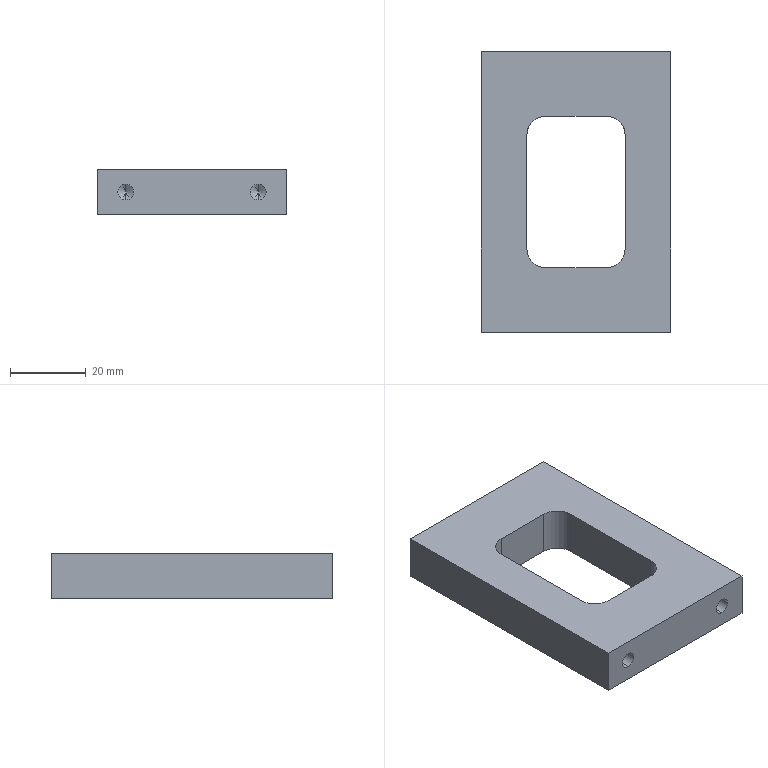Part | SolidWorks | features Extrusion 1, HoleWzd 1, ICE 1, MirrorPattern 1 | 1 solid | 30 faces | box 50 x 74 x 12 mm | volume 31467 mm3 | cylinder 12 | plane 10 | cone 8 | commonest cylinder face diameters 4.2 x8 10 x4
STEP:
#1=CARTESIAN_POINT('',(-17.5,24.6,-2.1));
#2=VERTEX_POINT('',#1);
#3=CARTESIAN_POINT('',(-17.5,24.6,2.1));
#4=VERTEX_POINT('',#3);
#5=CARTESIAN_POINT('',(-17.5,24.6,0.));
#6=DIRECTION('',(0.,1.,0.));
#7=DIRECTION('',(0.,0.,1.));
#8=AXIS2_PLACEMENT_3D('',#5,#6,#7);
#9=CIRCLE('',#8,2.1);
#10=EDGE_CURVE('',#2,#4,#9,.T.);
#11=ORIENTED_EDGE('',*,*,#10,.F.);
#12=CARTESIAN_POINT('',(-17.5,37.,-2.1));
#13=VERTEX_POINT('',#12);
#14=CARTESIAN_POINT('',(-17.5,37.,-2.1));
#15=DIRECTION('',(0.,1.,0.));
#16=VECTOR('',#15,1000.);
#17=LINE('',#14,#16);
#18=EDGE_CURVE('',#2,#13,#17,.T.);
#19=ORIENTED_EDGE('',*,*,#18,.T.);
#20=CARTESIAN_POINT('',(-17.5,37.,2.1));
#21=VERTEX_POINT('',#20);
#22=CARTESIAN_POINT('',(-17.5,37.,0.));
#23=DIRECTION('',(0.,1.,0.));
#24=DIRECTION('',(0.,0.,1.));
#25=AXIS2_PLACEMENT_3D('',#22,#23,#24);
#26=CIRCLE('',#25,2.1);
#27=EDGE_CURVE('',#13,#21,#26,.T.);
#28=ORIENTED_EDGE('',*,*,#27,.T.);
#29=CARTESIAN_POINT('',(-17.5,37.,2.1));
#30=DIRECTION('',(0.,1.,0.));
#31=VECTOR('',#30,1000.);
#32=LINE('',#29,#31);
#33=EDGE_CURVE('',#4,#21,#32,.T.);
#34=ORIENTED_EDGE('',*,*,#33,.F.);
#35=EDGE_LOOP('',(#11,#19,#28,#34));
#36=FACE_OUTER_BOUND('',#35,.T.);
#37=CARTESIAN_POINT('',(-17.5,37.,0.));
#38=DIRECTION('',(0.,1.,0.));
#39=DIRECTION('',(0.,0.,1.));
#40=AXIS2_PLACEMENT_3D('',#37,#38,#39);
#41=CYLINDRICAL_SURFACE('',#40,2.1);
#42=ADVANCED_FACE('',(#36),#41,.F.);
#43=CARTESIAN_POINT('',(-17.5,23.338,0.));
#44=VERTEX_POINT('',#43);
#45=CARTESIAN_POINT('',(-17.5,24.6,2.1));
#46=DIRECTION('',(0.,0.515,0.8572));
#47=VECTOR('',#46,1000.);
#48=LINE('',#45,#47);
#49=EDGE_CURVE('',#44,#4,#48,.T.);
#50=ORIENTED_EDGE('',*,*,#49,.F.);
#51=CARTESIAN_POINT('',(-17.5,24.6,-2.1));
#52=DIRECTION('',(0.,0.515,-0.8572));
#53=VECTOR('',#52,1000.);
#54=LINE('',#51,#53);
#55=EDGE_CURVE('',#44,#2,#54,.T.);
#56=ORIENTED_EDGE('',*,*,#55,.T.);
#57=ORIENTED_EDGE('',*,*,#10,.T.);
#58=EDGE_LOOP('',(#50,#56,#57));
#59=FACE_OUTER_BOUND('',#58,.T.);
#60=CARTESIAN_POINT('',(-17.5,24.6,0.));
#61=DIRECTION('',(0.,1.,0.));
#62=DIRECTION('',(0.,0.,1.));
#63=AXIS2_PLACEMENT_3D('',#60,#61,#62);
#64=CONICAL_SURFACE('',#63,2.1,1.03);
#65=ADVANCED_FACE('',(#59),#64,.F.);
#66=CARTESIAN_POINT('',(17.5,24.6,-2.1));
#67=VERTEX_POINT('',#66);
#68=CARTESIAN_POINT('',(17.5,24.6,2.1));
#69=VERTEX_POINT('',#68);
#70=CARTESIAN_POINT('',(17.5,24.6,0.));
#71=DIRECTION('',(0.,1.,0.));
#72=DIRECTION('',(0.,0.,1.));
#73=AXIS2_PLACEMENT_3D('',#70,#71,#72);
#74=CIRCLE('',#73,2.1);
#75=EDGE_CURVE('',#67,#69,#74,.T.);
#76=ORIENTED_EDGE('',*,*,#75,.F.);
#77=CARTESIAN_POINT('',(17.5,37.,-2.1));
#78=VERTEX_POINT('',#77);
#79=CARTESIAN_POINT('',(17.5,37.,-2.1));
#80=DIRECTION('',(0.,1.,0.));
#81=VECTOR('',#80,1000.);
#82=LINE('',#79,#81);
#83=EDGE_CURVE('',#67,#78,#82,.T.);
#84=ORIENTED_EDGE('',*,*,#83,.T.);
#85=CARTESIAN_POINT('',(17.5,37.,2.1));
#86=VERTEX_POINT('',#85);
#87=CARTESIAN_POINT('',(17.5,37.,0.));
#88=DIRECTION('',(0.,1.,0.));
#89=DIRECTION('',(0.,0.,1.));
#90=AXIS2_PLACEMENT_3D('',#87,#88,#89);
#91=CIRCLE('',#90,2.1);
#92=EDGE_CURVE('',#78,#86,#91,.T.);
#93=ORIENTED_EDGE('',*,*,#92,.T.);
#94=CARTESIAN_POINT('',(17.5,37.,2.1));
#95=DIRECTION('',(0.,1.,0.));
#96=VECTOR('',#95,1000.);
#97=LINE('',#94,#96);
#98=EDGE_CURVE('',#69,#86,#97,.T.);
#99=ORIENTED_EDGE('',*,*,#98,.F.);
#100=EDGE_LOOP('',(#76,#84,#93,#99));
#101=FACE_OUTER_BOUND('',#100,.T.);
#102=CARTESIAN_POINT('',(17.5,37.,0.));
#103=DIRECTION('',(0.,1.,0.));
#104=DIRECTION('',(0.,0.,1.));
#105=AXIS2_PLACEMENT_3D('',#102,#103,#104);
#106=CYLINDRICAL_SURFACE('',#105,2.1);
#107=ADVANCED_FACE('',(#101),#106,.F.);
#108=CARTESIAN_POINT('',(17.5,23.338,0.));
#109=VERTEX_POINT('',#108);
#110=CARTESIAN_POINT('',(17.5,24.6,2.1));
#111=DIRECTION('',(0.,0.515,0.8572));
#112=VECTOR('',#111,1000.);
#113=LINE('',#110,#112);
#114=EDGE_CURVE('',#109,#69,#113,.T.);
#115=ORIENTED_EDGE('',*,*,#114,.F.);
#116=CARTESIAN_POINT('',(17.5,24.6,-2.1));
#117=DIRECTION('',(0.,0.515,-0.8572));
#118=VECTOR('',#117,1000.);
#119=LINE('',#116,#118);
#120=EDGE_CURVE('',#109,#67,#119,.T.);
#121=ORIENTED_EDGE('',*,*,#120,.T.);
#122=ORIENTED_EDGE('',*,*,#75,.T.);
#123=EDGE_LOOP('',(#115,#121,#122));
#124=FACE_OUTER_BOUND('',#123,.T.);
#125=CARTESIAN_POINT('',(17.5,24.6,0.));
#126=DIRECTION('',(0.,1.,0.));
#127=DIRECTION('',(0.,0.,1.));
#128=AXIS2_PLACEMENT_3D('',#125,#126,#127);
#129=CONICAL_SURFACE('',#128,2.1,1.03);
#130=ADVANCED_FACE('',(#124),#129,.F.);
#131=CARTESIAN_POINT('',(-17.5,-24.6,2.1));
#132=VERTEX_POINT('',#131);
#133=CARTESIAN_POINT('',(-17.5,-24.6,-2.1));
#134=VERTEX_POINT('',#133);
#135=CARTESIAN_POINT('',(-17.5,-24.6,0.));
#136=DIRECTION('',(0.,-1.,0.));
#137=DIRECTION('',(0.,0.,-1.));
#138=AXIS2_PLACEMENT_3D('',#135,#136,#137);
#139=CIRCLE('',#138,2.1);
#140=EDGE_CURVE('',#132,#134,#139,.T.);
#141=ORIENTED_EDGE('',*,*,#140,.F.);
#142=CARTESIAN_POINT('',(-17.5,-37.,2.1));
#143=VERTEX_POINT('',#142);
#144=CARTESIAN_POINT('',(-17.5,-37.,2.1));
#145=DIRECTION('',(0.,-1.,0.));
#146=VECTOR('',#145,1000.);
#147=LINE('',#144,#146);
#148=EDGE_CURVE('',#132,#143,#147,.T.);
#149=ORIENTED_EDGE('',*,*,#148,.T.);
#150=CARTESIAN_POINT('',(-17.5,-37.,-2.1));
#151=VERTEX_POINT('',#150);
#152=CARTESIAN_POINT('',(-17.5,-37.,0.));
#153=DIRECTION('',(0.,-1.,0.));
#154=DIRECTION('',(0.,0.,-1.));
#155=AXIS2_PLACEMENT_3D('',#152,#153,#154);
#156=CIRCLE('',#155,2.1);
#157=EDGE_CURVE('',#143,#151,#156,.T.);
#158=ORIENTED_EDGE('',*,*,#157,.T.);
#159=CARTESIAN_POINT('',(-17.5,-37.,-2.1));
#160=DIRECTION('',(0.,-1.,0.));
#161=VECTOR('',#160,1000.);
#162=LINE('',#159,#161);
#163=EDGE_CURVE('',#134,#151,#162,.T.);
#164=ORIENTED_EDGE('',*,*,#163,.F.);
#165=EDGE_LOOP('',(#141,#149,#158,#164));
#166=FACE_OUTER_BOUND('',#165,.T.);
#167=CARTESIAN_POINT('',(-17.5,-37.,0.));
#168=DIRECTION('',(0.,-1.,0.));
#169=DIRECTION('',(0.,0.,-1.));
#170=AXIS2_PLACEMENT_3D('',#167,#168,#169);
#171=CYLINDRICAL_SURFACE('',#170,2.1);
#172=ADVANCED_FACE('',(#166),#171,.F.);
#173=CARTESIAN_POINT('',(-17.5,-23.338,0.));
#174=VERTEX_POINT('',#173);
#175=CARTESIAN_POINT('',(-17.5,-24.6,-2.1));
#176=DIRECTION('',(0.,-0.515,-0.8572));
#177=VECTOR('',#176,1000.);
#178=LINE('',#175,#177);
#179=EDGE_CURVE('',#174,#134,#178,.T.);
#180=ORIENTED_EDGE('',*,*,#179,.F.);
#181=CARTESIAN_POINT('',(-17.5,-24.6,2.1));
#182=DIRECTION('',(0.,-0.515,0.8572));
#183=VECTOR('',#182,1000.);
#184=LINE('',#181,#183);
#185=EDGE_CURVE('',#174,#132,#184,.T.);
#186=ORIENTED_EDGE('',*,*,#185,.T.);
#187=ORIENTED_EDGE('',*,*,#140,.T.);
#188=EDGE_LOOP('',(#180,#186,#187));
#189=FACE_OUTER_BOUND('',#188,.T.);
#190=CARTESIAN_POINT('',(-17.5,-24.6,0.));
#191=DIRECTION('',(0.,-1.,0.));
#192=DIRECTION('',(0.,0.,-1.));
#193=AXIS2_PLACEMENT_3D('',#190,#191,#192);
#194=CONICAL_SURFACE('',#193,2.1,1.03);
#195=ADVANCED_FACE('',(#189),#194,.F.);
#196=CARTESIAN_POINT('',(17.5,-24.6,2.1));
#197=VERTEX_POINT('',#196);
#198=CARTESIAN_POINT('',(17.5,-24.6,-2.1));
#199=VERTEX_POINT('',#198);
#200=CARTESIAN_POINT('',(17.5,-24.6,0.));
#201=DIRECTION('',(0.,-1.,0.));
#202=DIRECTION('',(0.,0.,-1.));
#203=AXIS2_PLACEMENT_3D('',#200,#201,#202);
#204=CIRCLE('',#203,2.1);
#205=EDGE_CURVE('',#197,#199,#204,.T.);
#206=ORIENTED_EDGE('',*,*,#205,.F.);
#207=CARTESIAN_POINT('',(17.5,-37.,2.1));
#208=VERTEX_POINT('',#207);
#209=CARTESIAN_POINT('',(17.5,-37.,2.1));
#210=DIRECTION('',(0.,-1.,0.));
#211=VECTOR('',#210,1000.);
#212=LINE('',#209,#211);
#213=EDGE_CURVE('',#197,#208,#212,.T.);
#214=ORIENTED_EDGE('',*,*,#213,.T.);
#215=CARTESIAN_POINT('',(17.5,-37.,-2.1));
#216=VERTEX_POINT('',#215);
#217=CARTESIAN_POINT('',(17.5,-37.,0.));
#218=DIRECTION('',(0.,-1.,0.));
#219=DIRECTION('',(0.,0.,-1.));
#220=AXIS2_PLACEMENT_3D('',#217,#218,#219);
#221=CIRCLE('',#220,2.1);
#222=EDGE_CURVE('',#208,#216,#221,.T.);
#223=ORIENTED_EDGE('',*,*,#222,.T.);
#224=CARTESIAN_POINT('',(17.5,-37.,-2.1));
#225=DIRECTION('',(0.,-1.,0.));
#226=VECTOR('',#225,1000.);
#227=LINE('',#224,#226);
#228=EDGE_CURVE('',#199,#216,#227,.T.);
#229=ORIENTED_EDGE('',*,*,#228,.F.);
#230=EDGE_LOOP('',(#206,#214,#223,#229));
#231=FACE_OUTER_BOUND('',#230,.T.);
#232=CARTESIAN_POINT('',(17.5,-37.,0.));
#233=DIRECTION('',(0.,-1.,0.));
#234=DIRECTION('',(0.,0.,-1.));
#235=AXIS2_PLACEMENT_3D('',#232,#233,#234);
#236=CYLINDRICAL_SURFACE('',#235,2.1);
#237=ADVANCED_FACE('',(#231),#236,.F.);
#238=CARTESIAN_POINT('',(17.5,-23.338,0.));
#239=VERTEX_POINT('',#238);
#240=CARTESIAN_POINT('',(17.5,-24.6,-2.1));
#241=DIRECTION('',(0.,-0.515,-0.8572));
#242=VECTOR('',#241,1000.);
#243=LINE('',#240,#242);
#244=EDGE_CURVE('',#239,#199,#243,.T.);
#245=ORIENTED_EDGE('',*,*,#244,.F.);
#246=CARTESIAN_POINT('',(17.5,-24.6,2.1));
#247=DIRECTION('',(0.,-0.515,0.8572));
#248=VECTOR('',#247,1000.);
#249=LINE('',#246,#248);
#250=EDGE_CURVE('',#239,#197,#249,.T.);
#251=ORIENTED_EDGE('',*,*,#250,.T.);
#252=ORIENTED_EDGE('',*,*,#205,.T.);
#253=EDGE_LOOP('',(#245,#251,#252));
#254=FACE_OUTER_BOUND('',#253,.T.);
#255=CARTESIAN_POINT('',(17.5,-24.6,0.));
#256=DIRECTION('',(0.,-1.,0.));
#257=DIRECTION('',(0.,0.,-1.));
#258=AXIS2_PLACEMENT_3D('',#255,#256,#257);
#259=CONICAL_SURFACE('',#258,2.1,1.03);
#260=ADVANCED_FACE('',(#254),#259,.F.);
#261=CARTESIAN_POINT('',(25.,-37.,-6.));
#262=VERTEX_POINT('',#261);
#263=CARTESIAN_POINT('',(25.,37.,-6.));
#264=VERTEX_POINT('',#263);
#265=CARTESIAN_POINT('',(25.,-37.,-6.));
#266=DIRECTION('',(0.,1.,0.));
#267=VECTOR('',#266,1000.);
#268=LINE('',#265,#267);
#269=EDGE_CURVE('',#262,#264,#268,.T.);
#270=ORIENTED_EDGE('',*,*,#269,.T.);
#271=CARTESIAN_POINT('',(25.,37.,6.));
#272=VERTEX_POINT('',#271);
#273=CARTESIAN_POINT('',(25.,37.,6.));
#274=DIRECTION('',(0.,0.,-1.));
#275=VECTOR('',#274,1000.);
#276=LINE('',#273,#275);
#277=EDGE_CURVE('',#272,#264,#276,.T.);
#278=ORIENTED_EDGE('',*,*,#277,.F.);
#279=CARTESIAN_POINT('',(25.,-37.,6.));
#280=VERTEX_POINT('',#279);
#281=CARTESIAN_POINT('',(25.,-37.,6.));
#282=DIRECTION('',(0.,1.,0.));
#283=VECTOR('',#282,1000.);
#284=LINE('',#281,#283);
#285=EDGE_CURVE('',#280,#272,#284,.T.);
#286=ORIENTED_EDGE('',*,*,#285,.F.);
#287=CARTESIAN_POINT('',(25.,-37.,6.));
#288=DIRECTION('',(0.,0.,-1.));
#289=VECTOR('',#288,1000.);
#290=LINE('',#287,#289);
#291=EDGE_CURVE('',#280,#262,#290,.T.);
#292=ORIENTED_EDGE('',*,*,#291,.T.);
#293=EDGE_LOOP('',(#270,#278,#286,#292));
#294=FACE_OUTER_BOUND('',#293,.T.);
#295=CARTESIAN_POINT('',(25.,-37.,6.));
#296=DIRECTION('',(-1.,0.,0.));
#297=DIRECTION('',(0.,0.,1.));
#298=AXIS2_PLACEMENT_3D('',#295,#296,#297);
#299=PLANE('',#298);
#300=ADVANCED_FACE('',(#294),#299,.F.);
#301=CARTESIAN_POINT('',(-17.5,37.,0.));
#302=DIRECTION('',(0.,1.,0.));
#303=DIRECTION('',(0.,0.,1.));
#304=AXIS2_PLACEMENT_3D('',#301,#302,#303);
#305=CIRCLE('',#304,2.1);
#306=EDGE_CURVE('',#21,#13,#305,.T.);
#307=ORIENTED_EDGE('',*,*,#306,.F.);
#308=ORIENTED_EDGE('',*,*,#27,.F.);
#309=EDGE_LOOP('',(#307,#308));
#310=FACE_BOUND('',#309,.T.);
#311=CARTESIAN_POINT('',(17.5,37.,0.));
#312=DIRECTION('',(0.,1.,0.));
#313=DIRECTION('',(0.,0.,1.));
#314=AXIS2_PLACEMENT_3D('',#311,#312,#313);
#315=CIRCLE('',#314,2.1);
#316=EDGE_CURVE('',#86,#78,#315,.T.);
#317=ORIENTED_EDGE('',*,*,#316,.F.);
#318=ORIENTED_EDGE('',*,*,#92,.F.);
#319=EDGE_LOOP('',(#317,#318));
#320=FACE_BOUND('',#319,.T.);
#321=CARTESIAN_POINT('',(-25.,37.,-6.));
#322=VERTEX_POINT('',#321);
#323=CARTESIAN_POINT('',(-25.,37.,-6.));
#324=DIRECTION('',(-1.,0.,0.));
#325=VECTOR('',#324,1000.);
#326=LINE('',#323,#325);
#327=EDGE_CURVE('',#264,#322,#326,.T.);
#328=ORIENTED_EDGE('',*,*,#327,.T.);
#329=CARTESIAN_POINT('',(-25.,37.,6.));
#330=VERTEX_POINT('',#329);
#331=CARTESIAN_POINT('',(-25.,37.,6.));
#332=DIRECTION('',(0.,0.,-1.));
#333=VECTOR('',#332,1000.);
#334=LINE('',#331,#333);
#335=EDGE_CURVE('',#330,#322,#334,.T.);
#336=ORIENTED_EDGE('',*,*,#335,.F.);
#337=CARTESIAN_POINT('',(-25.,37.,6.));
#338=DIRECTION('',(-1.,0.,0.));
#339=VECTOR('',#338,1000.);
#340=LINE('',#337,#339);
#341=EDGE_CURVE('',#272,#330,#340,.T.);
#342=ORIENTED_EDGE('',*,*,#341,.F.);
#343=ORIENTED_EDGE('',*,*,#277,.T.);
#344=EDGE_LOOP('',(#328,#336,#342,#343));
#345=FACE_OUTER_BOUND('',#344,.T.);
#346=CARTESIAN_POINT('',(-25.,37.,6.));
#347=DIRECTION('',(0.,-1.,0.));
#348=DIRECTION('',(0.,0.,-1.));
#349=AXIS2_PLACEMENT_3D('',#346,#347,#348);
#350=PLANE('',#349);
#351=ADVANCED_FACE('',(#310,#320,#345),#350,.F.);
#352=CARTESIAN_POINT('',(-25.,-37.,-6.));
#353=VERTEX_POINT('',#352);
#354=CARTESIAN_POINT('',(-25.,-37.,-6.));
#355=DIRECTION('',(0.,-1.,0.));
#356=VECTOR('',#355,1000.);
#357=LINE('',#354,#356);
#358=EDGE_CURVE('',#322,#353,#357,.T.);
#359=ORIENTED_EDGE('',*,*,#358,.T.);
#360=CARTESIAN_POINT('',(-25.,-37.,6.));
#361=VERTEX_POINT('',#360);
#362=CARTESIAN_POINT('',(-25.,-37.,6.));
#363=DIRECTION('',(0.,0.,-1.));
#364=VECTOR('',#363,1000.);
#365=LINE('',#362,#364);
#366=EDGE_CURVE('',#361,#353,#365,.T.);
#367=ORIENTED_EDGE('',*,*,#366,.F.);
#368=CARTESIAN_POINT('',(-25.,-37.,6.));
#369=DIRECTION('',(0.,-1.,0.));
#370=VECTOR('',#369,1000.);
#371=LINE('',#368,#370);
#372=EDGE_CURVE('',#330,#361,#371,.T.);
#373=ORIENTED_EDGE('',*,*,#372,.F.);
#374=ORIENTED_EDGE('',*,*,#335,.T.);
#375=EDGE_LOOP('',(#359,#367,#373,#374));
#376=FACE_OUTER_BOUND('',#375,.T.);
#377=CARTESIAN_POINT('',(-25.,-37.,6.));
#378=DIRECTION('',(1.,0.,0.));
#379=DIRECTION('',(0.,0.,-1.));
#380=AXIS2_PLACEMENT_3D('',#377,#378,#379);
#381=PLANE('',#380);
#382=ADVANCED_FACE('',(#376),#381,.F.);
#383=CARTESIAN_POINT('',(-17.5,-37.,0.));
#384=DIRECTION('',(0.,-1.,0.));
#385=DIRECTION('',(0.,0.,-1.));
#386=AXIS2_PLACEMENT_3D('',#383,#384,#385);
#387=CIRCLE('',#386,2.1);
#388=EDGE_CURVE('',#151,#143,#387,.T.);
#389=ORIENTED_EDGE('',*,*,#388,.F.);
#390=ORIENTED_EDGE('',*,*,#157,.F.);
#391=EDGE_LOOP('',(#389,#390));
#392=FACE_BOUND('',#391,.T.);
#393=CARTESIAN_POINT('',(17.5,-37.,0.));
#394=DIRECTION('',(0.,-1.,0.));
#395=DIRECTION('',(0.,0.,-1.));
#396=AXIS2_PLACEMENT_3D('',#393,#394,#395);
#397=CIRCLE('',#396,2.1);
#398=EDGE_CURVE('',#216,#208,#397,.T.);
#399=ORIENTED_EDGE('',*,*,#398,.F.);
#400=ORIENTED_EDGE('',*,*,#222,.F.);
#401=EDGE_LOOP('',(#399,#400));
#402=FACE_BOUND('',#401,.T.);
#403=CARTESIAN_POINT('',(-25.,-37.,-6.));
#404=DIRECTION('',(1.,0.,0.));
#405=VECTOR('',#404,1000.);
#406=LINE('',#403,#405);
#407=EDGE_CURVE('',#353,#262,#406,.T.);
#408=ORIENTED_EDGE('',*,*,#407,.T.);
#409=ORIENTED_EDGE('',*,*,#291,.F.);
#410=CARTESIAN_POINT('',(-25.,-37.,6.));
#411=DIRECTION('',(1.,0.,0.));
#412=VECTOR('',#411,1000.);
#413=LINE('',#410,#412);
#414=EDGE_CURVE('',#361,#280,#413,.T.);
#415=ORIENTED_EDGE('',*,*,#414,.F.);
#416=ORIENTED_EDGE('',*,*,#366,.T.);
#417=EDGE_LOOP('',(#408,#409,#415,#416));
#418=FACE_OUTER_BOUND('',#417,.T.);
#419=CARTESIAN_POINT('',(-25.,-37.,6.));
#420=DIRECTION('',(0.,1.,0.));
#421=DIRECTION('',(0.,0.,1.));
#422=AXIS2_PLACEMENT_3D('',#419,#420,#421);
#423=PLANE('',#422);
#424=ADVANCED_FACE('',(#392,#402,#418),#423,.F.);
#425=CARTESIAN_POINT('',(13.,-15.,6.));
#426=VERTEX_POINT('',#425);
#427=CARTESIAN_POINT('',(13.,15.,6.));
#428=VERTEX_POINT('',#427);
#429=CARTESIAN_POINT('',(13.,-15.,6.));
#430=DIRECTION('',(0.,1.,0.));
#431=VECTOR('',#430,1000.);
#432=LINE('',#429,#431);
#433=EDGE_CURVE('',#426,#428,#432,.T.);
#434=ORIENTED_EDGE('',*,*,#433,.F.);
#435=CARTESIAN_POINT('',(8.,-20.,6.));
#436=VERTEX_POINT('',#435);
#437=CARTESIAN_POINT('',(8.,-15.,6.));
#438=DIRECTION('',(0.,0.,1.));
#439=DIRECTION('',(1.,0.,0.));
#440=AXIS2_PLACEMENT_3D('',#437,#438,#439);
#441=CIRCLE('',#440,5.);
#442=EDGE_CURVE('',#436,#426,#441,.T.);
#443=ORIENTED_EDGE('',*,*,#442,.F.);
#444=CARTESIAN_POINT('',(-8.,-20.,6.));
#445=VERTEX_POINT('',#444);
#446=CARTESIAN_POINT('',(-8.,-20.,6.));
#447=DIRECTION('',(1.,0.,0.));
#448=VECTOR('',#447,1000.);
#449=LINE('',#446,#448);
#450=EDGE_CURVE('',#445,#436,#449,.T.);
#451=ORIENTED_EDGE('',*,*,#450,.F.);
#452=CARTESIAN_POINT('',(-13.,-15.,6.));
#453=VERTEX_POINT('',#452);
#454=CARTESIAN_POINT('',(-8.,-15.,6.));
#455=DIRECTION('',(0.,0.,1.));
#456=DIRECTION('',(-1.,0.,0.));
#457=AXIS2_PLACEMENT_3D('',#454,#455,#456);
#458=CIRCLE('',#457,5.);
#459=EDGE_CURVE('',#453,#445,#458,.T.);
#460=ORIENTED_EDGE('',*,*,#459,.F.);
#461=CARTESIAN_POINT('',(-13.,15.,6.));
#462=VERTEX_POINT('',#461);
#463=CARTESIAN_POINT('',(-13.,-15.,6.));
#464=DIRECTION('',(0.,-1.,0.));
#465=VECTOR('',#464,1000.);
#466=LINE('',#463,#465);
#467=EDGE_CURVE('',#462,#453,#466,.T.);
#468=ORIENTED_EDGE('',*,*,#467,.F.);
#469=CARTESIAN_POINT('',(-8.,20.,6.));
#470=VERTEX_POINT('',#469);
#471=CARTESIAN_POINT('',(-8.,15.,6.));
#472=DIRECTION('',(0.,0.,1.));
#473=DIRECTION('',(-1.,0.,0.));
#474=AXIS2_PLACEMENT_3D('',#471,#472,#473);
#475=CIRCLE('',#474,5.);
#476=EDGE_CURVE('',#470,#462,#475,.T.);
#477=ORIENTED_EDGE('',*,*,#476,.F.);
#478=CARTESIAN_POINT('',(8.,20.,6.));
#479=VERTEX_POINT('',#478);
#480=CARTESIAN_POINT('',(-8.,20.,6.));
#481=DIRECTION('',(-1.,0.,0.));
#482=VECTOR('',#481,1000.);
#483=LINE('',#480,#482);
#484=EDGE_CURVE('',#479,#470,#483,.T.);
#485=ORIENTED_EDGE('',*,*,#484,.F.);
#486=CARTESIAN_POINT('',(8.,15.,6.));
#487=DIRECTION('',(0.,0.,1.));
#488=DIRECTION('',(-1.,0.,0.));
#489=AXIS2_PLACEMENT_3D('',#486,#487,#488);
#490=CIRCLE('',#489,5.);
#491=EDGE_CURVE('',#428,#479,#490,.T.);
#492=ORIENTED_EDGE('',*,*,#491,.F.);
#493=EDGE_LOOP('',(#434,#443,#451,#460,#468,#477,#485,#492));
#494=FACE_BOUND('',#493,.T.);
#495=ORIENTED_EDGE('',*,*,#285,.T.);
#496=ORIENTED_EDGE('',*,*,#341,.T.);
#497=ORIENTED_EDGE('',*,*,#372,.T.);
#498=ORIENTED_EDGE('',*,*,#414,.T.);
#499=EDGE_LOOP('',(#495,#496,#497,#498));
#500=FACE_OUTER_BOUND('',#499,.T.);
#501=CARTESIAN_POINT('',(0.,0.,6.));
#502=DIRECTION('',(0.,0.,-1.));
#503=DIRECTION('',(-1.,0.,0.));
#504=AXIS2_PLACEMENT_3D('',#501,#502,#503);
#505=PLANE('',#504);
#506=ADVANCED_FACE('',(#494,#500),#505,.F.);
#507=CARTESIAN_POINT('',(8.,-20.,-6.));
#508=VERTEX_POINT('',#507);
#509=CARTESIAN_POINT('',(13.,-15.,-6.));
#510=VERTEX_POINT('',#509);
#511=CARTESIAN_POINT('',(8.,-15.,-6.));
#512=DIRECTION('',(0.,0.,1.));
#513=DIRECTION('',(1.,0.,0.));
#514=AXIS2_PLACEMENT_3D('',#511,#512,#513);
#515=CIRCLE('',#514,5.);
#516=EDGE_CURVE('',#508,#510,#515,.T.);
#517=ORIENTED_EDGE('',*,*,#516,.T.);
#518=CARTESIAN_POINT('',(13.,15.,-6.));
#519=VERTEX_POINT('',#518);
#520=CARTESIAN_POINT('',(13.,-15.,-6.));
#521=DIRECTION('',(0.,1.,0.));
#522=VECTOR('',#521,1000.);
#523=LINE('',#520,#522);
#524=EDGE_CURVE('',#510,#519,#523,.T.);
#525=ORIENTED_EDGE('',*,*,#524,.T.);
#526=CARTESIAN_POINT('',(8.,20.,-6.));
#527=VERTEX_POINT('',#526);
#528=CARTESIAN_POINT('',(8.,15.,-6.));
#529=DIRECTION('',(0.,0.,1.));
#530=DIRECTION('',(-1.,0.,0.));
#531=AXIS2_PLACEMENT_3D('',#528,#529,#530);
#532=CIRCLE('',#531,5.);
#533=EDGE_CURVE('',#519,#527,#532,.T.);
#534=ORIENTED_EDGE('',*,*,#533,.T.);
#535=CARTESIAN_POINT('',(-8.,20.,-6.));
#536=VERTEX_POINT('',#535);
#537=CARTESIAN_POINT('',(-8.,20.,-6.));
#538=DIRECTION('',(-1.,0.,0.));
#539=VECTOR('',#538,1000.);
#540=LINE('',#537,#539);
#541=EDGE_CURVE('',#527,#536,#540,.T.);
#542=ORIENTED_EDGE('',*,*,#541,.T.);
#543=CARTESIAN_POINT('',(-13.,15.,-6.));
#544=VERTEX_POINT('',#543);
#545=CARTESIAN_POINT('',(-8.,15.,-6.));
#546=DIRECTION('',(0.,0.,1.));
#547=DIRECTION('',(-1.,0.,0.));
#548=AXIS2_PLACEMENT_3D('',#545,#546,#547);
#549=CIRCLE('',#548,5.);
#550=EDGE_CURVE('',#536,#544,#549,.T.);
#551=ORIENTED_EDGE('',*,*,#550,.T.);
#552=CARTESIAN_POINT('',(-13.,-15.,-6.));
#553=VERTEX_POINT('',#552);
#554=CARTESIAN_POINT('',(-13.,-15.,-6.));
#555=DIRECTION('',(0.,-1.,0.));
#556=VECTOR('',#555,1000.);
#557=LINE('',#554,#556);
#558=EDGE_CURVE('',#544,#553,#557,.T.);
#559=ORIENTED_EDGE('',*,*,#558,.T.);
#560=CARTESIAN_POINT('',(-8.,-20.,-6.));
#561=VERTEX_POINT('',#560);
#562=CARTESIAN_POINT('',(-8.,-15.,-6.));
#563=DIRECTION('',(0.,0.,1.));
#564=DIRECTION('',(-1.,0.,0.));
#565=AXIS2_PLACEMENT_3D('',#562,#563,#564);
#566=CIRCLE('',#565,5.);
#567=EDGE_CURVE('',#553,#561,#566,.T.);
#568=ORIENTED_EDGE('',*,*,#567,.T.);
#569=CARTESIAN_POINT('',(-8.,-20.,-6.));
#570=DIRECTION('',(1.,0.,0.));
#571=VECTOR('',#570,1000.);
#572=LINE('',#569,#571);
#573=EDGE_CURVE('',#561,#508,#572,.T.);
#574=ORIENTED_EDGE('',*,*,#573,.T.);
#575=EDGE_LOOP('',(#517,#525,#534,#542,#551,#559,#568,#574));
#576=FACE_BOUND('',#575,.T.);
#577=ORIENTED_EDGE('',*,*,#269,.F.);
#578=ORIENTED_EDGE('',*,*,#407,.F.);
#579=ORIENTED_EDGE('',*,*,#358,.F.);
#580=ORIENTED_EDGE('',*,*,#327,.F.);
#581=EDGE_LOOP('',(#577,#578,#579,#580));
#582=FACE_OUTER_BOUND('',#581,.T.);
#583=CARTESIAN_POINT('',(0.,0.,-6.));
#584=DIRECTION('',(0.,0.,-1.));
#585=DIRECTION('',(-1.,0.,0.));
#586=AXIS2_PLACEMENT_3D('',#583,#584,#585);
#587=PLANE('',#586);
#588=ADVANCED_FACE('',(#576,#582),#587,.T.);
#589=ORIENTED_EDGE('',*,*,#250,.F.);
#590=ORIENTED_EDGE('',*,*,#244,.T.);
#591=CARTESIAN_POINT('',(17.5,-24.6,0.));
#592=DIRECTION('',(0.,-1.,0.));
#593=DIRECTION('',(0.,0.,-1.));
#594=AXIS2_PLACEMENT_3D('',#591,#592,#593);
#595=CIRCLE('',#594,2.1);
#596=EDGE_CURVE('',#199,#197,#595,.T.);
#597=ORIENTED_EDGE('',*,*,#596,.T.);
#598=EDGE_LOOP('',(#589,#590,#597));
#599=FACE_OUTER_BOUND('',#598,.T.);
#600=CARTESIAN_POINT('',(17.5,-24.6,0.));
#601=DIRECTION('',(0.,-1.,0.));
#602=DIRECTION('',(0.,0.,-1.));
#603=AXIS2_PLACEMENT_3D('',#600,#601,#602);
#604=CONICAL_SURFACE('',#603,2.1,1.03);
#605=ADVANCED_FACE('',(#599),#604,.F.);
#606=ORIENTED_EDGE('',*,*,#213,.F.);
#607=ORIENTED_EDGE('',*,*,#596,.F.);
#608=ORIENTED_EDGE('',*,*,#228,.T.);
#609=ORIENTED_EDGE('',*,*,#398,.T.);
#610=EDGE_LOOP('',(#606,#607,#608,#609));
#611=FACE_OUTER_BOUND('',#610,.T.);
#612=CARTESIAN_POINT('',(17.5,-37.,0.));
#613=DIRECTION('',(0.,-1.,0.));
#614=DIRECTION('',(0.,0.,-1.));
#615=AXIS2_PLACEMENT_3D('',#612,#613,#614);
#616=CYLINDRICAL_SURFACE('',#615,2.1);
#617=ADVANCED_FACE('',(#611),#616,.F.);
#618=ORIENTED_EDGE('',*,*,#185,.F.);
#619=ORIENTED_EDGE('',*,*,#179,.T.);
#620=CARTESIAN_POINT('',(-17.5,-24.6,0.));
#621=DIRECTION('',(0.,-1.,0.));
#622=DIRECTION('',(0.,0.,-1.));
#623=AXIS2_PLACEMENT_3D('',#620,#621,#622);
#624=CIRCLE('',#623,2.1);
#625=EDGE_CURVE('',#134,#132,#624,.T.);
#626=ORIENTED_EDGE('',*,*,#625,.T.);
#627=EDGE_LOOP('',(#618,#619,#626));
#628=FACE_OUTER_BOUND('',#627,.T.);
#629=CARTESIAN_POINT('',(-17.5,-24.6,0.));
#630=DIRECTION('',(0.,-1.,0.));
#631=DIRECTION('',(0.,0.,-1.));
#632=AXIS2_PLACEMENT_3D('',#629,#630,#631);
#633=CONICAL_SURFACE('',#632,2.1,1.03);
#634=ADVANCED_FACE('',(#628),#633,.F.);
#635=ORIENTED_EDGE('',*,*,#148,.F.);
#636=ORIENTED_EDGE('',*,*,#625,.F.);
#637=ORIENTED_EDGE('',*,*,#163,.T.);
#638=ORIENTED_EDGE('',*,*,#388,.T.);
#639=EDGE_LOOP('',(#635,#636,#637,#638));
#640=FACE_OUTER_BOUND('',#639,.T.);
#641=CARTESIAN_POINT('',(-17.5,-37.,0.));
#642=DIRECTION('',(0.,-1.,0.));
#643=DIRECTION('',(0.,0.,-1.));
#644=AXIS2_PLACEMENT_3D('',#641,#642,#643);
#645=CYLINDRICAL_SURFACE('',#644,2.1);
#646=ADVANCED_FACE('',(#640),#645,.F.);
#647=ORIENTED_EDGE('',*,*,#120,.F.);
#648=ORIENTED_EDGE('',*,*,#114,.T.);
#649=CARTESIAN_POINT('',(17.5,24.6,0.));
#650=DIRECTION('',(0.,1.,0.));
#651=DIRECTION('',(0.,0.,1.));
#652=AXIS2_PLACEMENT_3D('',#649,#650,#651);
#653=CIRCLE('',#652,2.1);
#654=EDGE_CURVE('',#69,#67,#653,.T.);
#655=ORIENTED_EDGE('',*,*,#654,.T.);
#656=EDGE_LOOP('',(#647,#648,#655));
#657=FACE_OUTER_BOUND('',#656,.T.);
#658=CARTESIAN_POINT('',(17.5,24.6,0.));
#659=DIRECTION('',(0.,1.,0.));
#660=DIRECTION('',(0.,0.,1.));
#661=AXIS2_PLACEMENT_3D('',#658,#659,#660);
#662=CONICAL_SURFACE('',#661,2.1,1.03);
#663=ADVANCED_FACE('',(#657),#662,.F.);
#664=ORIENTED_EDGE('',*,*,#83,.F.);
#665=ORIENTED_EDGE('',*,*,#654,.F.);
#666=ORIENTED_EDGE('',*,*,#98,.T.);
#667=ORIENTED_EDGE('',*,*,#316,.T.);
#668=EDGE_LOOP('',(#664,#665,#666,#667));
#669=FACE_OUTER_BOUND('',#668,.T.);
#670=CARTESIAN_POINT('',(17.5,37.,0.));
#671=DIRECTION('',(0.,1.,0.));
#672=DIRECTION('',(0.,0.,1.));
#673=AXIS2_PLACEMENT_3D('',#670,#671,#672);
#674=CYLINDRICAL_SURFACE('',#673,2.1);
#675=ADVANCED_FACE('',(#669),#674,.F.);
#676=ORIENTED_EDGE('',*,*,#55,.F.);
#677=ORIENTED_EDGE('',*,*,#49,.T.);
#678=CARTESIAN_POINT('',(-17.5,24.6,0.));
#679=DIRECTION('',(0.,1.,0.));
#680=DIRECTION('',(0.,0.,1.));
#681=AXIS2_PLACEMENT_3D('',#678,#679,#680);
#682=CIRCLE('',#681,2.1);
#683=EDGE_CURVE('',#4,#2,#682,.T.);
#684=ORIENTED_EDGE('',*,*,#683,.T.);
#685=EDGE_LOOP('',(#676,#677,#684));
#686=FACE_OUTER_BOUND('',#685,.T.);
#687=CARTESIAN_POINT('',(-17.5,24.6,0.));
#688=DIRECTION('',(0.,1.,0.));
#689=DIRECTION('',(0.,0.,1.));
#690=AXIS2_PLACEMENT_3D('',#687,#688,#689);
#691=CONICAL_SURFACE('',#690,2.1,1.03);
#692=ADVANCED_FACE('',(#686),#691,.F.);
#693=ORIENTED_EDGE('',*,*,#18,.F.);
#694=ORIENTED_EDGE('',*,*,#683,.F.);
#695=ORIENTED_EDGE('',*,*,#33,.T.);
#696=ORIENTED_EDGE('',*,*,#306,.T.);
#697=EDGE_LOOP('',(#693,#694,#695,#696));
#698=FACE_OUTER_BOUND('',#697,.T.);
#699=CARTESIAN_POINT('',(-17.5,37.,0.));
#700=DIRECTION('',(0.,1.,0.));
#701=DIRECTION('',(0.,0.,1.));
#702=AXIS2_PLACEMENT_3D('',#699,#700,#701);
#703=CYLINDRICAL_SURFACE('',#702,2.1);
#704=ADVANCED_FACE('',(#698),#703,.F.);
#705=ORIENTED_EDGE('',*,*,#442,.T.);
#706=CARTESIAN_POINT('',(13.,-15.,-6.));
#707=DIRECTION('',(0.,0.,1.));
#708=VECTOR('',#707,1000.);
#709=LINE('',#706,#708);
#710=EDGE_CURVE('',#510,#426,#709,.T.);
#711=ORIENTED_EDGE('',*,*,#710,.F.);
#712=ORIENTED_EDGE('',*,*,#516,.F.);
#713=CARTESIAN_POINT('',(8.,-20.,-6.));
#714=DIRECTION('',(0.,0.,1.));
#715=VECTOR('',#714,1000.);
#716=LINE('',#713,#715);
#717=EDGE_CURVE('',#508,#436,#716,.T.);
#718=ORIENTED_EDGE('',*,*,#717,.T.);
#719=EDGE_LOOP('',(#705,#711,#712,#718));
#720=FACE_OUTER_BOUND('',#719,.T.);
#721=CARTESIAN_POINT('',(8.,-15.,-6.));
#722=DIRECTION('',(0.,0.,1.));
#723=DIRECTION('',(1.,0.,0.));
#724=AXIS2_PLACEMENT_3D('',#721,#722,#723);
#725=CYLINDRICAL_SURFACE('',#724,5.);
#726=ADVANCED_FACE('',(#720),#725,.F.);
#727=ORIENTED_EDGE('',*,*,#450,.T.);
#728=ORIENTED_EDGE('',*,*,#717,.F.);
#729=ORIENTED_EDGE('',*,*,#573,.F.);
#730=CARTESIAN_POINT('',(-8.,-20.,-6.));
#731=DIRECTION('',(0.,0.,1.));
#732=VECTOR('',#731,1000.);
#733=LINE('',#730,#732);
#734=EDGE_CURVE('',#561,#445,#733,.T.);
#735=ORIENTED_EDGE('',*,*,#734,.T.);
#736=EDGE_LOOP('',(#727,#728,#729,#735));
#737=FACE_OUTER_BOUND('',#736,.T.);
#738=CARTESIAN_POINT('',(-8.,-20.,-6.));
#739=DIRECTION('',(0.,-1.,0.));
#740=DIRECTION('',(0.,0.,-1.));
#741=AXIS2_PLACEMENT_3D('',#738,#739,#740);
#742=PLANE('',#741);
#743=ADVANCED_FACE('',(#737),#742,.F.);
#744=ORIENTED_EDGE('',*,*,#459,.T.);
#745=ORIENTED_EDGE('',*,*,#734,.F.);
#746=ORIENTED_EDGE('',*,*,#567,.F.);
#747=CARTESIAN_POINT('',(-13.,-15.,-6.));
#748=DIRECTION('',(0.,0.,1.));
#749=VECTOR('',#748,1000.);
#750=LINE('',#747,#749);
#751=EDGE_CURVE('',#553,#453,#750,.T.);
#752=ORIENTED_EDGE('',*,*,#751,.T.);
#753=EDGE_LOOP('',(#744,#745,#746,#752));
#754=FACE_OUTER_BOUND('',#753,.T.);
#755=CARTESIAN_POINT('',(-8.,-15.,-6.));
#756=DIRECTION('',(0.,0.,1.));
#757=DIRECTION('',(1.,0.,0.));
#758=AXIS2_PLACEMENT_3D('',#755,#756,#757);
#759=CYLINDRICAL_SURFACE('',#758,5.);
#760=ADVANCED_FACE('',(#754),#759,.F.);
#761=ORIENTED_EDGE('',*,*,#467,.T.);
#762=ORIENTED_EDGE('',*,*,#751,.F.);
#763=ORIENTED_EDGE('',*,*,#558,.F.);
#764=CARTESIAN_POINT('',(-13.,15.,-6.));
#765=DIRECTION('',(0.,0.,1.));
#766=VECTOR('',#765,1000.);
#767=LINE('',#764,#766);
#768=EDGE_CURVE('',#544,#462,#767,.T.);
#769=ORIENTED_EDGE('',*,*,#768,.T.);
#770=EDGE_LOOP('',(#761,#762,#763,#769));
#771=FACE_OUTER_BOUND('',#770,.T.);
#772=CARTESIAN_POINT('',(-13.,-15.,-6.));
#773=DIRECTION('',(-1.,0.,0.));
#774=DIRECTION('',(0.,0.,1.));
#775=AXIS2_PLACEMENT_3D('',#772,#773,#774);
#776=PLANE('',#775);
#777=ADVANCED_FACE('',(#771),#776,.F.);
#778=ORIENTED_EDGE('',*,*,#476,.T.);
#779=ORIENTED_EDGE('',*,*,#768,.F.);
#780=ORIENTED_EDGE('',*,*,#550,.F.);
#781=CARTESIAN_POINT('',(-8.,20.,-6.));
#782=DIRECTION('',(0.,0.,1.));
#783=VECTOR('',#782,1000.);
#784=LINE('',#781,#783);
#785=EDGE_CURVE('',#536,#470,#784,.T.);
#786=ORIENTED_EDGE('',*,*,#785,.T.);
#787=EDGE_LOOP('',(#778,#779,#780,#786));
#788=FACE_OUTER_BOUND('',#787,.T.);
#789=CARTESIAN_POINT('',(-8.,15.,-6.));
#790=DIRECTION('',(0.,0.,1.));
#791=DIRECTION('',(1.,0.,0.));
#792=AXIS2_PLACEMENT_3D('',#789,#790,#791);
#793=CYLINDRICAL_SURFACE('',#792,5.);
#794=ADVANCED_FACE('',(#788),#793,.F.);
#795=ORIENTED_EDGE('',*,*,#484,.T.);
#796=ORIENTED_EDGE('',*,*,#785,.F.);
#797=ORIENTED_EDGE('',*,*,#541,.F.);
#798=CARTESIAN_POINT('',(8.,20.,-6.));
#799=DIRECTION('',(0.,0.,1.));
#800=VECTOR('',#799,1000.);
#801=LINE('',#798,#800);
#802=EDGE_CURVE('',#527,#479,#801,.T.);
#803=ORIENTED_EDGE('',*,*,#802,.T.);
#804=EDGE_LOOP('',(#795,#796,#797,#803));
#805=FACE_OUTER_BOUND('',#804,.T.);
#806=CARTESIAN_POINT('',(-8.,20.,-6.));
#807=DIRECTION('',(0.,1.,0.));
#808=DIRECTION('',(0.,0.,1.));
#809=AXIS2_PLACEMENT_3D('',#806,#807,#808);
#810=PLANE('',#809);
#811=ADVANCED_FACE('',(#805),#810,.F.);
#812=ORIENTED_EDGE('',*,*,#491,.T.);
#813=ORIENTED_EDGE('',*,*,#802,.F.);
#814=ORIENTED_EDGE('',*,*,#533,.F.);
#815=CARTESIAN_POINT('',(13.,15.,-6.));
#816=DIRECTION('',(0.,0.,1.));
#817=VECTOR('',#816,1000.);
#818=LINE('',#815,#817);
#819=EDGE_CURVE('',#519,#428,#818,.T.);
#820=ORIENTED_EDGE('',*,*,#819,.T.);
#821=EDGE_LOOP('',(#812,#813,#814,#820));
#822=FACE_OUTER_BOUND('',#821,.T.);
#823=CARTESIAN_POINT('',(8.,15.,-6.));
#824=DIRECTION('',(0.,0.,1.));
#825=DIRECTION('',(1.,0.,0.));
#826=AXIS2_PLACEMENT_3D('',#823,#824,#825);
#827=CYLINDRICAL_SURFACE('',#826,5.);
#828=ADVANCED_FACE('',(#822),#827,.F.);
#829=ORIENTED_EDGE('',*,*,#433,.T.);
#830=ORIENTED_EDGE('',*,*,#819,.F.);
#831=ORIENTED_EDGE('',*,*,#524,.F.);
#832=ORIENTED_EDGE('',*,*,#710,.T.);
#833=EDGE_LOOP('',(#829,#830,#831,#832));
#834=FACE_OUTER_BOUND('',#833,.T.);
#835=CARTESIAN_POINT('',(13.,-15.,-6.));
#836=DIRECTION('',(1.,0.,0.));
#837=DIRECTION('',(0.,0.,-1.));
#838=AXIS2_PLACEMENT_3D('',#835,#836,#837);
#839=PLANE('',#838);
#840=ADVANCED_FACE('',(#834),#839,.F.);
#841=CLOSED_SHELL('',(#42,#65,#107,#130,#172,#195,#237,#260,#300,#351,#382,#424,#506,#588,#605,#617,#634,#646,#663,#675,#692,#704,#726,#743,#760,#777,#794,#811,#828,#840));
#842=MANIFOLD_SOLID_BREP('',#841);
#843=CARTESIAN_POINT('',(0.,0.,0.));
#844=DIRECTION('',(0.,0.,1.));
#845=DIRECTION('',(1.,0.,0.));
#846=AXIS2_PLACEMENT_3D('',#843,#844,#845);
#847=(LENGTH_UNIT()NAMED_UNIT(*)SI_UNIT(.MILLI.,.METRE.));
#848=UNCERTAINTY_MEASURE_WITH_UNIT(LENGTH_MEASURE(0.00001),#847,'','');
#849=(NAMED_UNIT(*)PLANE_ANGLE_UNIT()SI_UNIT($,.RADIAN.));
#850=(NAMED_UNIT(*)SI_UNIT($,.STERADIAN.)SOLID_ANGLE_UNIT());
#851=(GEOMETRIC_REPRESENTATION_CONTEXT(3)GLOBAL_UNCERTAINTY_ASSIGNED_CONTEXT((#848))GLOBAL_UNIT_ASSIGNED_CONTEXT((#847,#849,#850))REPRESENTATION_CONTEXT('',''));
#852=ADVANCED_BREP_SHAPE_REPRESENTATION('',(#842,#846),#851);